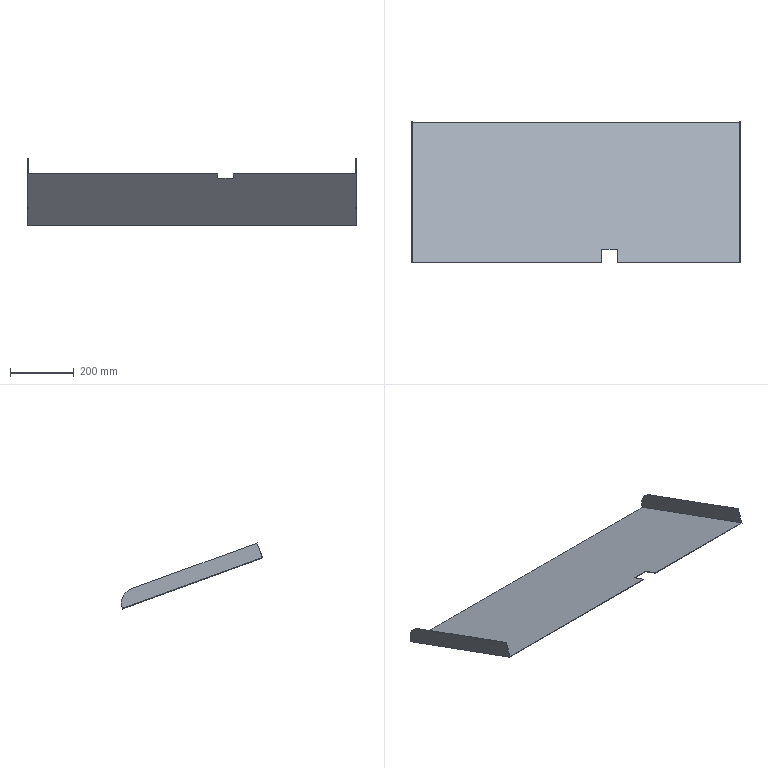Part | NX | features solid 2 | 1 solid | 16 faces | box 1030 x 443.096 x 207.161 mm | volume 1047311 mm3 | plane 14 | cylinder 2 | commonest cylinder face diameters 100 x2
STEP:
#1=CARTESIAN_POINT('',(-655.,759.919,-518.224));
#2=VERTEX_POINT('',#1);
#3=CARTESIAN_POINT('',(-60.,759.919,-518.224));
#4=VERTEX_POINT('',#3);
#5=CARTESIAN_POINT('',(-608.,759.919,-518.224));
#6=DIRECTION('',(1.,0.,0.));
#7=VECTOR('',#6,1000.);
#8=LINE('',#5,#7);
#9=EDGE_CURVE('',#2,#4,#8,.T.);
#10=ORIENTED_EDGE('',*,*,#9,.T.);
#11=CARTESIAN_POINT('',(-60.,760.603,-516.345));
#12=VERTEX_POINT('',#11);
#13=CARTESIAN_POINT('',(-60.,760.603,-516.345));
#14=DIRECTION('',(0.,-0.342,-0.9397));
#15=VECTOR('',#14,1000.);
#16=LINE('',#13,#15);
#17=EDGE_CURVE('',#4,#12,#16,.F.);
#18=ORIENTED_EDGE('',*,*,#17,.T.);
#19=CARTESIAN_POINT('',(-653.,760.603,-516.345));
#20=VERTEX_POINT('',#19);
#21=CARTESIAN_POINT('',(-608.,760.603,-516.345));
#22=DIRECTION('',(1.,0.,0.));
#23=VECTOR('',#22,1000.);
#24=LINE('',#21,#23);
#25=EDGE_CURVE('',#20,#12,#24,.T.);
#26=ORIENTED_EDGE('',*,*,#25,.F.);
#27=CARTESIAN_POINT('',(-653.,777.02,-471.24));
#28=VERTEX_POINT('',#27);
#29=CARTESIAN_POINT('',(-653.,760.603,-516.345));
#30=DIRECTION('',(0.,0.342,0.9397));
#31=VECTOR('',#30,1000.);
#32=LINE('',#29,#31);
#33=EDGE_CURVE('',#20,#28,#32,.T.);
#34=ORIENTED_EDGE('',*,*,#33,.T.);
#35=CARTESIAN_POINT('',(-655.,777.02,-471.24));
#36=VERTEX_POINT('',#35);
#37=CARTESIAN_POINT('',(-620.,777.02,-471.24));
#38=DIRECTION('',(-1.,0.,0.));
#39=VECTOR('',#38,1000.);
#40=LINE('',#37,#39);
#41=EDGE_CURVE('',#36,#28,#40,.F.);
#42=ORIENTED_EDGE('',*,*,#41,.F.);
#43=CARTESIAN_POINT('',(-655.,760.603,-516.345));
#44=DIRECTION('',(0.,0.342,0.9397));
#45=VECTOR('',#44,1000.);
#46=LINE('',#43,#45);
#47=EDGE_CURVE('',#36,#2,#46,.F.);
#48=ORIENTED_EDGE('',*,*,#47,.T.);
#49=EDGE_LOOP('',(#10,#18,#26,#34,#42,#48));
#50=FACE_BOUND('',#49,.T.);
#51=CARTESIAN_POINT('',(-608.,760.603,-516.345));
#52=DIRECTION('',(0.,0.9397,-0.342));
#53=DIRECTION('',(1.,0.,0.));
#54=AXIS2_PLACEMENT_3D('',#51,#52,#53);
#55=PLANE('',#54);
#56=ADVANCED_FACE('',(#50),#55,.F.);
#57=CARTESIAN_POINT('',(-653.,1200.,-676.272));
#58=VERTEX_POINT('',#57);
#59=CARTESIAN_POINT('',(-653.,1200.,-678.401));
#60=VERTEX_POINT('',#59);
#61=CARTESIAN_POINT('',(-653.,1200.,-700.));
#62=DIRECTION('',(0.,0.,-1.));
#63=VECTOR('',#62,1000.);
#64=LINE('',#61,#63);
#65=EDGE_CURVE('',#58,#60,#64,.T.);
#66=ORIENTED_EDGE('',*,*,#65,.F.);
#67=CARTESIAN_POINT('',(373.,1200.,-676.272));
#68=VERTEX_POINT('',#67);
#69=CARTESIAN_POINT('',(-1915.,1200.,-676.272));
#70=DIRECTION('',(1.,0.,0.));
#71=VECTOR('',#70,1000.);
#72=LINE('',#69,#71);
#73=EDGE_CURVE('',#58,#68,#72,.T.);
#74=ORIENTED_EDGE('',*,*,#73,.T.);
#75=CARTESIAN_POINT('',(373.,1200.,-678.401));
#76=VERTEX_POINT('',#75);
#77=CARTESIAN_POINT('',(373.,1200.,-700.));
#78=DIRECTION('',(0.,0.,-1.));
#79=VECTOR('',#78,1000.);
#80=LINE('',#77,#79);
#81=EDGE_CURVE('',#68,#76,#80,.T.);
#82=ORIENTED_EDGE('',*,*,#81,.T.);
#83=CARTESIAN_POINT('',(-1915.,1200.,-678.401));
#84=DIRECTION('',(1.,0.,0.));
#85=VECTOR('',#84,1000.);
#86=LINE('',#83,#85);
#87=EDGE_CURVE('',#60,#76,#86,.T.);
#88=ORIENTED_EDGE('',*,*,#87,.F.);
#89=EDGE_LOOP('',(#66,#74,#82,#88));
#90=FACE_BOUND('',#89,.T.);
#91=CARTESIAN_POINT('',(-1915.,1200.,-700.));
#92=DIRECTION('',(0.,-1.,0.));
#93=DIRECTION('',(-1.,0.,0.));
#94=AXIS2_PLACEMENT_3D('',#91,#92,#93);
#95=PLANE('',#94);
#96=ADVANCED_FACE('',(#90),#95,.F.);
#97=ORIENTED_EDGE('',*,*,#25,.T.);
#98=CARTESIAN_POINT('',(-60.,801.917,-531.382));
#99=VERTEX_POINT('',#98);
#100=CARTESIAN_POINT('',(-60.,1286.831,-707.876));
#101=DIRECTION('',(0.,-0.9397,0.342));
#102=VECTOR('',#101,1000.);
#103=LINE('',#100,#102);
#104=EDGE_CURVE('',#12,#99,#103,.F.);
#105=ORIENTED_EDGE('',*,*,#104,.T.);
#106=CARTESIAN_POINT('',(-10.,801.917,-531.382));
#107=VERTEX_POINT('',#106);
#108=CARTESIAN_POINT('',(-608.,801.917,-531.382));
#109=DIRECTION('',(-1.,0.,0.));
#110=VECTOR('',#109,1000.);
#111=LINE('',#108,#110);
#112=EDGE_CURVE('',#99,#107,#111,.F.);
#113=ORIENTED_EDGE('',*,*,#112,.T.);
#114=CARTESIAN_POINT('',(-10.,760.603,-516.345));
#115=VERTEX_POINT('',#114);
#116=CARTESIAN_POINT('',(-10.,1286.831,-707.876));
#117=DIRECTION('',(0.,-0.9397,0.342));
#118=VECTOR('',#117,1000.);
#119=LINE('',#116,#118);
#120=EDGE_CURVE('',#107,#115,#119,.T.);
#121=ORIENTED_EDGE('',*,*,#120,.T.);
#122=CARTESIAN_POINT('',(373.,760.603,-516.345));
#123=VERTEX_POINT('',#122);
#124=CARTESIAN_POINT('',(-608.,760.603,-516.345));
#125=DIRECTION('',(1.,0.,0.));
#126=VECTOR('',#125,1000.);
#127=LINE('',#124,#126);
#128=EDGE_CURVE('',#115,#123,#127,.T.);
#129=ORIENTED_EDGE('',*,*,#128,.T.);
#130=CARTESIAN_POINT('',(373.,1286.831,-707.876));
#131=DIRECTION('',(0.,0.9397,-0.342));
#132=VECTOR('',#131,1000.);
#133=LINE('',#130,#132);
#134=EDGE_CURVE('',#123,#68,#133,.T.);
#135=ORIENTED_EDGE('',*,*,#134,.T.);
#136=ORIENTED_EDGE('',*,*,#73,.F.);
#137=CARTESIAN_POINT('',(-653.,1286.831,-707.876));
#138=DIRECTION('',(0.,0.9397,-0.342));
#139=VECTOR('',#138,1000.);
#140=LINE('',#137,#139);
#141=EDGE_CURVE('',#20,#58,#140,.T.);
#142=ORIENTED_EDGE('',*,*,#141,.F.);
#143=EDGE_LOOP('',(#97,#105,#113,#121,#129,#135,#136,#142));
#144=FACE_BOUND('',#143,.T.);
#145=CARTESIAN_POINT('',(-608.,1286.831,-707.876));
#146=DIRECTION('',(0.,-0.342,-0.9397));
#147=DIRECTION('',(-1.,0.,0.));
#148=AXIS2_PLACEMENT_3D('',#145,#146,#147);
#149=PLANE('',#148);
#150=ADVANCED_FACE('',(#144),#149,.F.);
#151=CARTESIAN_POINT('',(-655.,1170.116,-614.315));
#152=VERTEX_POINT('',#151);
#153=CARTESIAN_POINT('',(-655.,1200.,-678.401));
#154=VERTEX_POINT('',#153);
#155=CARTESIAN_POINT('',(-655.,1153.015,-661.3));
#156=DIRECTION('',(-1.,0.,0.));
#157=DIRECTION('',(0.,0.,1.));
#158=AXIS2_PLACEMENT_3D('',#155,#156,#157);
#159=CIRCLE('',#158,50.);
#160=EDGE_CURVE('',#152,#154,#159,.T.);
#161=ORIENTED_EDGE('',*,*,#160,.T.);
#162=CARTESIAN_POINT('',(-655.,1286.147,-709.755));
#163=DIRECTION('',(0.,0.9397,-0.342));
#164=VECTOR('',#163,1000.);
#165=LINE('',#162,#164);
#166=EDGE_CURVE('',#154,#2,#165,.F.);
#167=ORIENTED_EDGE('',*,*,#166,.T.);
#168=ORIENTED_EDGE('',*,*,#47,.F.);
#169=CARTESIAN_POINT('',(-655.,-1236.749,261.713));
#170=DIRECTION('',(0.,-0.9397,0.342));
#171=VECTOR('',#170,1000.);
#172=LINE('',#169,#171);
#173=EDGE_CURVE('',#152,#36,#172,.T.);
#174=ORIENTED_EDGE('',*,*,#173,.F.);
#175=EDGE_LOOP('',(#161,#167,#168,#174));
#176=FACE_BOUND('',#175,.T.);
#177=CARTESIAN_POINT('',(-655.,-1078.132,697.509));
#178=DIRECTION('',(-1.,0.,0.));
#179=DIRECTION('',(0.,0.342,0.9397));
#180=AXIS2_PLACEMENT_3D('',#177,#178,#179);
#181=PLANE('',#180);
#182=ADVANCED_FACE('',(#176),#181,.T.);
#183=ORIENTED_EDGE('',*,*,#128,.F.);
#184=CARTESIAN_POINT('',(-10.,759.919,-518.224));
#185=VERTEX_POINT('',#184);
#186=CARTESIAN_POINT('',(-10.,760.603,-516.345));
#187=DIRECTION('',(0.,-0.342,-0.9397));
#188=VECTOR('',#187,1000.);
#189=LINE('',#186,#188);
#190=EDGE_CURVE('',#115,#185,#189,.T.);
#191=ORIENTED_EDGE('',*,*,#190,.T.);
#192=CARTESIAN_POINT('',(375.,759.919,-518.224));
#193=VERTEX_POINT('',#192);
#194=CARTESIAN_POINT('',(-608.,759.919,-518.224));
#195=DIRECTION('',(1.,0.,0.));
#196=VECTOR('',#195,1000.);
#197=LINE('',#194,#196);
#198=EDGE_CURVE('',#185,#193,#197,.T.);
#199=ORIENTED_EDGE('',*,*,#198,.T.);
#200=CARTESIAN_POINT('',(375.,777.02,-471.24));
#201=VERTEX_POINT('',#200);
#202=CARTESIAN_POINT('',(375.,716.012,-638.858));
#203=DIRECTION('',(0.,0.342,0.9397));
#204=VECTOR('',#203,1000.);
#205=LINE('',#202,#204);
#206=EDGE_CURVE('',#201,#193,#205,.F.);
#207=ORIENTED_EDGE('',*,*,#206,.F.);
#208=CARTESIAN_POINT('',(373.,777.02,-471.24));
#209=VERTEX_POINT('',#208);
#210=CARTESIAN_POINT('',(230.,777.02,-471.24));
#211=DIRECTION('',(1.,0.,0.));
#212=VECTOR('',#211,1000.);
#213=LINE('',#210,#212);
#214=EDGE_CURVE('',#201,#209,#213,.F.);
#215=ORIENTED_EDGE('',*,*,#214,.T.);
#216=CARTESIAN_POINT('',(373.,760.603,-516.345));
#217=DIRECTION('',(0.,0.342,0.9397));
#218=VECTOR('',#217,1000.);
#219=LINE('',#216,#218);
#220=EDGE_CURVE('',#123,#209,#219,.T.);
#221=ORIENTED_EDGE('',*,*,#220,.F.);
#222=EDGE_LOOP('',(#183,#191,#199,#207,#215,#221));
#223=FACE_BOUND('',#222,.T.);
#224=CARTESIAN_POINT('',(-608.,760.603,-516.345));
#225=DIRECTION('',(0.,0.9397,-0.342));
#226=DIRECTION('',(1.,0.,0.));
#227=AXIS2_PLACEMENT_3D('',#224,#225,#226);
#228=PLANE('',#227);
#229=ADVANCED_FACE('',(#223),#228,.F.);
#230=CARTESIAN_POINT('',(375.,1200.,-678.401));
#231=VERTEX_POINT('',#230);
#232=CARTESIAN_POINT('',(375.,1179.052,-670.776));
#233=DIRECTION('',(0.,0.9397,-0.342));
#234=VECTOR('',#233,1000.);
#235=LINE('',#232,#234);
#236=EDGE_CURVE('',#231,#193,#235,.F.);
#237=ORIENTED_EDGE('',*,*,#236,.F.);
#238=CARTESIAN_POINT('',(375.,1170.116,-614.315));
#239=VERTEX_POINT('',#238);
#240=CARTESIAN_POINT('',(375.,1153.015,-661.3));
#241=DIRECTION('',(1.,0.,0.));
#242=DIRECTION('',(0.,0.,-1.));
#243=AXIS2_PLACEMENT_3D('',#240,#241,#242);
#244=CIRCLE('',#243,50.);
#245=EDGE_CURVE('',#231,#239,#244,.T.);
#246=ORIENTED_EDGE('',*,*,#245,.T.);
#247=CARTESIAN_POINT('',(375.,1196.153,-623.791));
#248=DIRECTION('',(0.,0.9397,-0.342));
#249=VECTOR('',#248,1000.);
#250=LINE('',#247,#249);
#251=EDGE_CURVE('',#239,#201,#250,.F.);
#252=ORIENTED_EDGE('',*,*,#251,.T.);
#253=ORIENTED_EDGE('',*,*,#206,.T.);
#254=EDGE_LOOP('',(#237,#246,#252,#253));
#255=FACE_BOUND('',#254,.T.);
#256=CARTESIAN_POINT('',(375.,1135.145,-791.41));
#257=DIRECTION('',(1.,0.,0.));
#258=DIRECTION('',(0.,-0.342,-0.9397));
#259=AXIS2_PLACEMENT_3D('',#256,#257,#258);
#260=PLANE('',#259);
#261=ADVANCED_FACE('',(#255),#260,.T.);
#262=CARTESIAN_POINT('',(-60.,802.474,-533.713));
#263=VERTEX_POINT('',#262);
#264=CARTESIAN_POINT('',(-60.,1286.147,-709.755));
#265=DIRECTION('',(0.,-0.9397,0.342));
#266=VECTOR('',#265,1000.);
#267=LINE('',#264,#266);
#268=EDGE_CURVE('',#4,#263,#267,.F.);
#269=ORIENTED_EDGE('',*,*,#268,.F.);
#270=ORIENTED_EDGE('',*,*,#9,.F.);
#271=ORIENTED_EDGE('',*,*,#166,.F.);
#272=CARTESIAN_POINT('',(-1915.,1200.,-678.401));
#273=DIRECTION('',(1.,0.,0.));
#274=VECTOR('',#273,1000.);
#275=LINE('',#272,#274);
#276=EDGE_CURVE('',#154,#60,#275,.T.);
#277=ORIENTED_EDGE('',*,*,#276,.T.);
#278=ORIENTED_EDGE('',*,*,#87,.T.);
#279=CARTESIAN_POINT('',(230.,1200.,-678.401));
#280=DIRECTION('',(1.,0.,0.));
#281=VECTOR('',#280,1000.);
#282=LINE('',#279,#281);
#283=EDGE_CURVE('',#231,#76,#282,.F.);
#284=ORIENTED_EDGE('',*,*,#283,.F.);
#285=ORIENTED_EDGE('',*,*,#236,.T.);
#286=ORIENTED_EDGE('',*,*,#198,.F.);
#287=CARTESIAN_POINT('',(-10.,802.474,-533.713));
#288=VERTEX_POINT('',#287);
#289=CARTESIAN_POINT('',(-10.,1286.147,-709.755));
#290=DIRECTION('',(0.,-0.9397,0.342));
#291=VECTOR('',#290,1000.);
#292=LINE('',#289,#291);
#293=EDGE_CURVE('',#288,#185,#292,.T.);
#294=ORIENTED_EDGE('',*,*,#293,.F.);
#295=CARTESIAN_POINT('',(-608.,802.474,-533.713));
#296=DIRECTION('',(-1.,0.,0.));
#297=VECTOR('',#296,1000.);
#298=LINE('',#295,#297);
#299=EDGE_CURVE('',#263,#288,#298,.F.);
#300=ORIENTED_EDGE('',*,*,#299,.F.);
#301=EDGE_LOOP('',(#269,#270,#271,#277,#278,#284,#285,#286,#294,#300));
#302=FACE_BOUND('',#301,.T.);
#303=CARTESIAN_POINT('',(-608.,1286.147,-709.755));
#304=DIRECTION('',(0.,-0.342,-0.9397));
#305=DIRECTION('',(-1.,0.,0.));
#306=AXIS2_PLACEMENT_3D('',#303,#304,#305);
#307=PLANE('',#306);
#308=ADVANCED_FACE('',(#302),#307,.T.);
#309=ORIENTED_EDGE('',*,*,#81,.F.);
#310=ORIENTED_EDGE('',*,*,#134,.F.);
#311=ORIENTED_EDGE('',*,*,#220,.T.);
#312=CARTESIAN_POINT('',(373.,1170.116,-614.315));
#313=VERTEX_POINT('',#312);
#314=CARTESIAN_POINT('',(373.,1217.101,-631.416));
#315=DIRECTION('',(0.,-0.9397,0.342));
#316=VECTOR('',#315,1000.);
#317=LINE('',#314,#316);
#318=EDGE_CURVE('',#313,#209,#317,.T.);
#319=ORIENTED_EDGE('',*,*,#318,.F.);
#320=CARTESIAN_POINT('',(373.,1153.015,-661.3));
#321=DIRECTION('',(-1.,0.,0.));
#322=DIRECTION('',(0.,0.,1.));
#323=AXIS2_PLACEMENT_3D('',#320,#321,#322);
#324=CIRCLE('',#323,50.);
#325=EDGE_CURVE('',#313,#76,#324,.T.);
#326=ORIENTED_EDGE('',*,*,#325,.T.);
#327=EDGE_LOOP('',(#309,#310,#311,#319,#326));
#328=FACE_BOUND('',#327,.T.);
#329=CARTESIAN_POINT('',(373.,1200.,-678.401));
#330=DIRECTION('',(-1.,0.,0.));
#331=DIRECTION('',(0.,0.,1.));
#332=AXIS2_PLACEMENT_3D('',#329,#330,#331);
#333=PLANE('',#332);
#334=ADVANCED_FACE('',(#328),#333,.T.);
#335=ORIENTED_EDGE('',*,*,#251,.F.);
#336=CARTESIAN_POINT('',(230.,1170.116,-614.315));
#337=DIRECTION('',(-1.,0.,0.));
#338=VECTOR('',#337,1000.);
#339=LINE('',#336,#338);
#340=EDGE_CURVE('',#239,#313,#339,.T.);
#341=ORIENTED_EDGE('',*,*,#340,.T.);
#342=ORIENTED_EDGE('',*,*,#318,.T.);
#343=ORIENTED_EDGE('',*,*,#214,.F.);
#344=EDGE_LOOP('',(#335,#341,#342,#343));
#345=FACE_BOUND('',#344,.T.);
#346=CARTESIAN_POINT('',(230.,1217.101,-631.416));
#347=DIRECTION('',(0.,-0.342,-0.9397));
#348=DIRECTION('',(0.,-0.9397,0.342));
#349=AXIS2_PLACEMENT_3D('',#346,#347,#348);
#350=PLANE('',#349);
#351=ADVANCED_FACE('',(#345),#350,.F.);
#352=ORIENTED_EDGE('',*,*,#245,.F.);
#353=ORIENTED_EDGE('',*,*,#283,.T.);
#354=ORIENTED_EDGE('',*,*,#325,.F.);
#355=ORIENTED_EDGE('',*,*,#340,.F.);
#356=EDGE_LOOP('',(#352,#353,#354,#355));
#357=FACE_BOUND('',#356,.T.);
#358=CARTESIAN_POINT('',(230.,1153.015,-661.3));
#359=DIRECTION('',(-1.,0.,0.));
#360=DIRECTION('',(0.,0.,1.));
#361=AXIS2_PLACEMENT_3D('',#358,#359,#360);
#362=CYLINDRICAL_SURFACE('',#361,50.);
#363=ADVANCED_FACE('',(#357),#362,.T.);
#364=ORIENTED_EDGE('',*,*,#141,.T.);
#365=ORIENTED_EDGE('',*,*,#65,.T.);
#366=CARTESIAN_POINT('',(-653.,1170.116,-614.315));
#367=VERTEX_POINT('',#366);
#368=CARTESIAN_POINT('',(-653.,1153.015,-661.3));
#369=DIRECTION('',(-1.,0.,0.));
#370=DIRECTION('',(0.,0.,1.));
#371=AXIS2_PLACEMENT_3D('',#368,#369,#370);
#372=CIRCLE('',#371,50.);
#373=EDGE_CURVE('',#60,#367,#372,.F.);
#374=ORIENTED_EDGE('',*,*,#373,.T.);
#375=CARTESIAN_POINT('',(-653.,1217.101,-631.416));
#376=DIRECTION('',(0.,0.9397,-0.342));
#377=VECTOR('',#376,1000.);
#378=LINE('',#375,#377);
#379=EDGE_CURVE('',#367,#28,#378,.F.);
#380=ORIENTED_EDGE('',*,*,#379,.T.);
#381=ORIENTED_EDGE('',*,*,#33,.F.);
#382=EDGE_LOOP('',(#364,#365,#374,#380,#381));
#383=FACE_BOUND('',#382,.T.);
#384=CARTESIAN_POINT('',(-653.,1200.,-678.401));
#385=DIRECTION('',(-1.,0.,0.));
#386=DIRECTION('',(0.,0.,1.));
#387=AXIS2_PLACEMENT_3D('',#384,#385,#386);
#388=PLANE('',#387);
#389=ADVANCED_FACE('',(#383),#388,.F.);
#390=ORIENTED_EDGE('',*,*,#379,.F.);
#391=CARTESIAN_POINT('',(-620.,1170.116,-614.315));
#392=DIRECTION('',(-1.,0.,0.));
#393=VECTOR('',#392,1000.);
#394=LINE('',#391,#393);
#395=EDGE_CURVE('',#367,#152,#394,.T.);
#396=ORIENTED_EDGE('',*,*,#395,.T.);
#397=ORIENTED_EDGE('',*,*,#173,.T.);
#398=ORIENTED_EDGE('',*,*,#41,.T.);
#399=EDGE_LOOP('',(#390,#396,#397,#398));
#400=FACE_BOUND('',#399,.T.);
#401=CARTESIAN_POINT('',(-620.,1217.101,-631.416));
#402=DIRECTION('',(0.,-0.342,-0.9397));
#403=DIRECTION('',(0.,-0.9397,0.342));
#404=AXIS2_PLACEMENT_3D('',#401,#402,#403);
#405=PLANE('',#404);
#406=ADVANCED_FACE('',(#400),#405,.F.);
#407=ORIENTED_EDGE('',*,*,#160,.F.);
#408=ORIENTED_EDGE('',*,*,#395,.F.);
#409=ORIENTED_EDGE('',*,*,#373,.F.);
#410=ORIENTED_EDGE('',*,*,#276,.F.);
#411=EDGE_LOOP('',(#407,#408,#409,#410));
#412=FACE_BOUND('',#411,.T.);
#413=CARTESIAN_POINT('',(-620.,1153.015,-661.3));
#414=DIRECTION('',(1.,0.,0.));
#415=DIRECTION('',(0.,0.,-1.));
#416=AXIS2_PLACEMENT_3D('',#413,#414,#415);
#417=CYLINDRICAL_SURFACE('',#416,50.);
#418=ADVANCED_FACE('',(#412),#417,.T.);
#419=ORIENTED_EDGE('',*,*,#17,.F.);
#420=ORIENTED_EDGE('',*,*,#268,.T.);
#421=CARTESIAN_POINT('',(-60.,699.909,-104.804));
#422=DIRECTION('',(0.,0.2326,-0.9726));
#423=VECTOR('',#422,1000.);
#424=LINE('',#421,#423);
#425=EDGE_CURVE('',#99,#263,#424,.T.);
#426=ORIENTED_EDGE('',*,*,#425,.F.);
#427=ORIENTED_EDGE('',*,*,#104,.F.);
#428=EDGE_LOOP('',(#419,#420,#426,#427));
#429=FACE_BOUND('',#428,.T.);
#430=CARTESIAN_POINT('',(-60.,720.,-100.));
#431=DIRECTION('',(1.,0.,0.));
#432=DIRECTION('',(0.,0.,-1.));
#433=AXIS2_PLACEMENT_3D('',#430,#431,#432);
#434=PLANE('',#433);
#435=ADVANCED_FACE('',(#429),#434,.T.);
#436=CARTESIAN_POINT('',(-10.,699.909,-104.804));
#437=DIRECTION('',(0.,0.2326,-0.9726));
#438=VECTOR('',#437,1000.);
#439=LINE('',#436,#438);
#440=EDGE_CURVE('',#288,#107,#439,.F.);
#441=ORIENTED_EDGE('',*,*,#440,.F.);
#442=ORIENTED_EDGE('',*,*,#293,.T.);
#443=ORIENTED_EDGE('',*,*,#190,.F.);
#444=ORIENTED_EDGE('',*,*,#120,.F.);
#445=EDGE_LOOP('',(#441,#442,#443,#444));
#446=FACE_BOUND('',#445,.T.);
#447=CARTESIAN_POINT('',(-10.,720.,-100.));
#448=DIRECTION('',(1.,0.,0.));
#449=DIRECTION('',(0.,0.,-1.));
#450=AXIS2_PLACEMENT_3D('',#447,#448,#449);
#451=PLANE('',#450);
#452=ADVANCED_FACE('',(#446),#451,.F.);
#453=ORIENTED_EDGE('',*,*,#425,.T.);
#454=ORIENTED_EDGE('',*,*,#299,.T.);
#455=ORIENTED_EDGE('',*,*,#440,.T.);
#456=ORIENTED_EDGE('',*,*,#112,.F.);
#457=EDGE_LOOP('',(#453,#454,#455,#456));
#458=FACE_BOUND('',#457,.T.);
#459=CARTESIAN_POINT('',(-20.,719.726,-187.674));
#460=DIRECTION('',(0.,-0.9726,-0.2326));
#461=DIRECTION('',(0.,0.2326,-0.9726));
#462=AXIS2_PLACEMENT_3D('',#459,#460,#461);
#463=PLANE('',#462);
#464=ADVANCED_FACE('',(#458),#463,.T.);
#465=CLOSED_SHELL('',(#56,#96,#150,#182,#229,#261,#308,#334,#351,#363,#389,#406,#418,#435,#452,#464));
#466=MANIFOLD_SOLID_BREP('',#465);
#467=(LENGTH_UNIT()NAMED_UNIT(*)SI_UNIT(.MILLI.,.METRE.));
#468=UNCERTAINTY_MEASURE_WITH_UNIT(LENGTH_MEASURE(0.00001),#467,'','');
#469=(NAMED_UNIT(*)PLANE_ANGLE_UNIT()SI_UNIT($,.RADIAN.));
#470=(NAMED_UNIT(*)SI_UNIT($,.STERADIAN.)SOLID_ANGLE_UNIT());
#471=(GEOMETRIC_REPRESENTATION_CONTEXT(3)GLOBAL_UNCERTAINTY_ASSIGNED_CONTEXT((#468))GLOBAL_UNIT_ASSIGNED_CONTEXT((#467,#469,#470))REPRESENTATION_CONTEXT('',''));
#472=ADVANCED_BREP_SHAPE_REPRESENTATION('',(#466),#471);